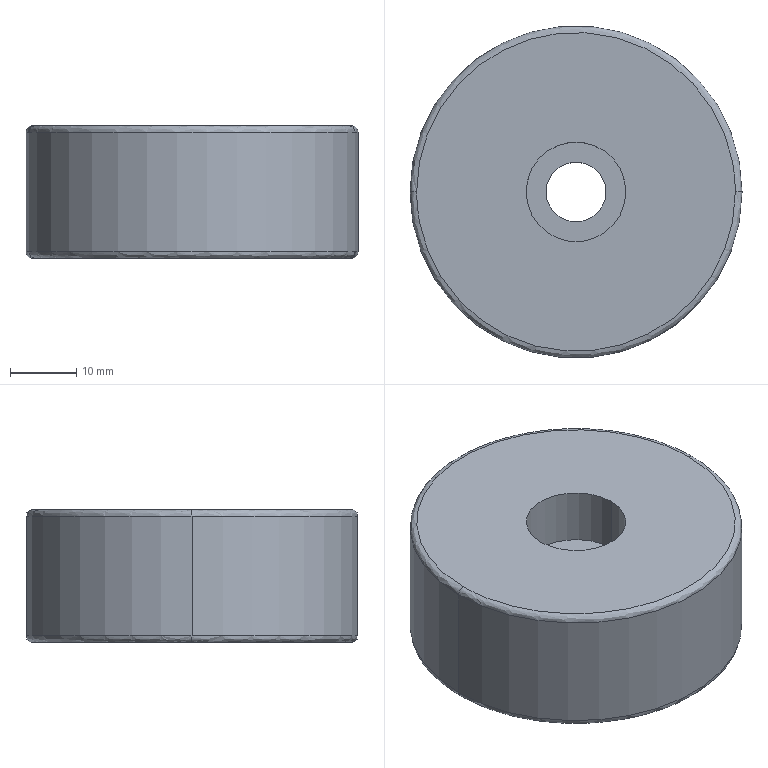Part | STEP file | Hard stop block | 1 solid | 13 faces | box 50 x 50 x 20 mm | volume 36960 mm3 | cylinder 6 | spline 4 | plane 3 | commonest cylinder face diameters 9 x2 15 x2 50 x2
STEP:
#1=CARTESIAN_POINT('',(0.,0.,0.));
#2=DIRECTION('',(0.,0.,1.));
#3=DIRECTION('',(1.,0.,0.));
#4=AXIS2_PLACEMENT_3D('',#1,#2,#3);
#5=CARTESIAN_POINT('',(25.,0.,1.));
#6=VERTEX_POINT('',#5);
#7=CARTESIAN_POINT('',(-25.,0.,1.));
#8=VERTEX_POINT('',#7);
#9=CARTESIAN_POINT('',(0.,0.,1.));
#10=DIRECTION('',(0.,0.,-1.));
#11=DIRECTION('',(1.,0.,0.));
#12=AXIS2_PLACEMENT_3D('',#9,#10,#11);
#13=CIRCLE('',#12,25.);
#14=CARTESIAN_POINT('',(-25.,0.,1.));
#15=CARTESIAN_POINT('',(-25.,-50.,1.));
#16=CARTESIAN_POINT('',(25.,-50.,1.));
#17=CARTESIAN_POINT('',(25.,0.,1.));
#18=CARTESIAN_POINT('',(-25.,0.,0.4142));
#19=CARTESIAN_POINT('',(-25.,-50.,0.4142));
#20=CARTESIAN_POINT('',(25.,-50.,0.4142));
#21=CARTESIAN_POINT('',(25.,0.,0.4142));
#22=CARTESIAN_POINT('',(-24.586,0.,0.));
#23=CARTESIAN_POINT('',(-24.586,-49.172,0.));
#24=CARTESIAN_POINT('',(24.586,-49.172,0.));
#25=CARTESIAN_POINT('',(24.586,0.,0.));
#26=CARTESIAN_POINT('',(-24.,0.,0.));
#27=CARTESIAN_POINT('',(-24.,-48.,0.));
#28=CARTESIAN_POINT('',(24.,-48.,0.));
#29=CARTESIAN_POINT('',(24.,0.,0.));
#30=(BOUNDED_SURFACE()B_SPLINE_SURFACE(3,3,((#14,#15,#16,#17),(#18,#19,#20,#21),(#22,#23,#24,#25),(#26,#27,#28,#29)),.UNSPECIFIED.,.F.,.F.,.F.)B_SPLINE_SURFACE_WITH_KNOTS((4,4),(4,4),(0.,1.),(0.,1.),.PIECEWISE_BEZIER_KNOTS.)GEOMETRIC_REPRESENTATION_ITEM()RATIONAL_B_SPLINE_SURFACE(((1.,0.3333,0.3333,1.),(0.8047,0.2682,0.2682,0.8047),(0.8047,0.2682,0.2682,0.8047),(1.,0.3333,0.3333,1.)))REPRESENTATION_ITEM('')SURFACE());
#31=CARTESIAN_POINT('',(0.,1.));
#32=CARTESIAN_POINT('',(0.,0.9763));
#33=CARTESIAN_POINT('',(0.,0.9319));
#34=CARTESIAN_POINT('',(0.,0.8733));
#35=CARTESIAN_POINT('',(0.,0.8206));
#36=CARTESIAN_POINT('',(0.,0.7724));
#37=CARTESIAN_POINT('',(0.,0.7279));
#38=CARTESIAN_POINT('',(0.,0.6861));
#39=CARTESIAN_POINT('',(0.,0.6465));
#40=CARTESIAN_POINT('',(0.,0.6086));
#41=CARTESIAN_POINT('',(0.,0.5718));
#42=CARTESIAN_POINT('',(0.,0.5357));
#43=CARTESIAN_POINT('',(0.,0.5));
#44=CARTESIAN_POINT('',(0.,0.4643));
#45=CARTESIAN_POINT('',(0.,0.4282));
#46=CARTESIAN_POINT('',(0.,0.3914));
#47=CARTESIAN_POINT('',(0.,0.3535));
#48=CARTESIAN_POINT('',(0.,0.3139));
#49=CARTESIAN_POINT('',(0.,0.2721));
#50=CARTESIAN_POINT('',(0.,0.2276));
#51=CARTESIAN_POINT('',(0.,0.1794));
#52=CARTESIAN_POINT('',(0.,0.1267));
#53=CARTESIAN_POINT('',(0.,0.06805));
#54=CARTESIAN_POINT('',(0.,0.02375));
#55=CARTESIAN_POINT('',(0.,0.));
#56=B_SPLINE_CURVE_WITH_KNOTS('',3,(#31,#32,#33,#34,#35,#36,#37,#38,#39,#40,#41,#42,#43,#44,#45,#46,#47,#48,#49,#50,#51,#52,#53,#54,#55),.UNSPECIFIED.,.F.,.F.,(4,1,1,1,1,1,1,1,1,1,1,1,1,1,1,1,1,1,1,1,1,1,4),(0.,0.1428,0.2856,0.4284,0.5712,0.714,0.8568,0.9996,1.142,1.285,1.428,1.571,1.714,1.856,1.999,2.142,2.285,2.428,2.57,2.713,2.856,2.999,3.142),.QUASI_UNIFORM_KNOTS.);
#57=(GEOMETRIC_REPRESENTATION_CONTEXT(2)PARAMETRIC_REPRESENTATION_CONTEXT()REPRESENTATION_CONTEXT('',''));
#58=DEFINITIONAL_REPRESENTATION('',(#56),#57);
#59=PCURVE('',#30,#58);
#60=CARTESIAN_POINT('',(0.,0.,20.));
#61=DIRECTION('',(0.,0.,-1.));
#62=DIRECTION('',(-1.,0.,0.));
#63=AXIS2_PLACEMENT_3D('',#60,#61,#62);
#64=CYLINDRICAL_SURFACE('',#63,25.);
#65=CARTESIAN_POINT('',(3.142,19.));
#66=DIRECTION('',(1.,0.));
#67=VECTOR('',#66,1.);
#68=LINE('',#65,#67);
#69=(GEOMETRIC_REPRESENTATION_CONTEXT(2)PARAMETRIC_REPRESENTATION_CONTEXT()REPRESENTATION_CONTEXT('',''));
#70=DEFINITIONAL_REPRESENTATION('',(#68),#69);
#71=PCURVE('',#64,#70);
#72=SURFACE_CURVE('',#13,(#59,#71),.PCURVE_S1.);
#73=EDGE_CURVE('',#6,#8,#72,.T.);
#74=ORIENTED_EDGE('',*,*,#73,.T.);
#75=CARTESIAN_POINT('',(-24.,0.,0.));
#76=VERTEX_POINT('',#75);
#77=CARTESIAN_POINT('',(-24.,0.,1.));
#78=DIRECTION('',(0.,-1.,0.));
#79=DIRECTION('',(-1.,0.,0.));
#80=AXIS2_PLACEMENT_3D('',#77,#78,#79);
#81=CIRCLE('',#80,1.);
#82=CARTESIAN_POINT('',(0.,0.));
#83=CARTESIAN_POINT('',(0.01683,0.));
#84=CARTESIAN_POINT('',(0.04999,0.));
#85=CARTESIAN_POINT('',(0.09843,0.));
#86=CARTESIAN_POINT('',(0.1457,0.));
#87=CARTESIAN_POINT('',(0.192,0.));
#88=CARTESIAN_POINT('',(0.2375,0.));
#89=CARTESIAN_POINT('',(0.2823,0.));
#90=CARTESIAN_POINT('',(0.3265,0.));
#91=CARTESIAN_POINT('',(0.3703,0.));
#92=CARTESIAN_POINT('',(0.4137,0.));
#93=CARTESIAN_POINT('',(0.4569,0.));
#94=CARTESIAN_POINT('',(0.5,0.));
#95=CARTESIAN_POINT('',(0.5431,0.));
#96=CARTESIAN_POINT('',(0.5863,0.));
#97=CARTESIAN_POINT('',(0.6297,0.));
#98=CARTESIAN_POINT('',(0.6735,0.));
#99=CARTESIAN_POINT('',(0.7177,0.));
#100=CARTESIAN_POINT('',(0.7625,0.));
#101=CARTESIAN_POINT('',(0.808,0.));
#102=CARTESIAN_POINT('',(0.8543,0.));
#103=CARTESIAN_POINT('',(0.9016,0.));
#104=CARTESIAN_POINT('',(0.95,0.));
#105=CARTESIAN_POINT('',(0.9832,0.));
#106=CARTESIAN_POINT('',(1.,0.));
#107=B_SPLINE_CURVE_WITH_KNOTS('',3,(#82,#83,#84,#85,#86,#87,#88,#89,#90,#91,#92,#93,#94,#95,#96,#97,#98,#99,#100,#101,#102,#103,#104,#105,#106),.UNSPECIFIED.,.F.,.F.,(4,1,1,1,1,1,1,1,1,1,1,1,1,1,1,1,1,1,1,1,1,1,4),(0.,0.0714,0.1428,0.2142,0.2856,0.357,0.4284,0.4998,0.5712,0.6426,0.714,0.7854,0.8568,0.9282,0.9996,1.071,1.142,1.214,1.285,1.357,1.428,1.499,1.571),.QUASI_UNIFORM_KNOTS.);
#108=(GEOMETRIC_REPRESENTATION_CONTEXT(2)PARAMETRIC_REPRESENTATION_CONTEXT()REPRESENTATION_CONTEXT('',''));
#109=DEFINITIONAL_REPRESENTATION('',(#107),#108);
#110=PCURVE('',#30,#109);
#111=CARTESIAN_POINT('',(25.,0.,1.));
#112=CARTESIAN_POINT('',(25.,50.,1.));
#113=CARTESIAN_POINT('',(-25.,50.,1.));
#114=CARTESIAN_POINT('',(-25.,0.,1.));
#115=CARTESIAN_POINT('',(25.,0.,0.4142));
#116=CARTESIAN_POINT('',(25.,50.,0.4142));
#117=CARTESIAN_POINT('',(-25.,50.,0.4142));
#118=CARTESIAN_POINT('',(-25.,0.,0.4142));
#119=CARTESIAN_POINT('',(24.586,0.,0.));
#120=CARTESIAN_POINT('',(24.586,49.172,0.));
#121=CARTESIAN_POINT('',(-24.586,49.172,0.));
#122=CARTESIAN_POINT('',(-24.586,0.,0.));
#123=CARTESIAN_POINT('',(24.,0.,0.));
#124=CARTESIAN_POINT('',(24.,48.,0.));
#125=CARTESIAN_POINT('',(-24.,48.,0.));
#126=CARTESIAN_POINT('',(-24.,0.,0.));
#127=(BOUNDED_SURFACE()B_SPLINE_SURFACE(3,3,((#111,#112,#113,#114),(#115,#116,#117,#118),(#119,#120,#121,#122),(#123,#124,#125,#126)),.UNSPECIFIED.,.F.,.F.,.F.)B_SPLINE_SURFACE_WITH_KNOTS((4,4),(4,4),(0.,1.),(0.,1.),.PIECEWISE_BEZIER_KNOTS.)GEOMETRIC_REPRESENTATION_ITEM()RATIONAL_B_SPLINE_SURFACE(((1.,0.3333,0.3333,1.),(0.8047,0.2682,0.2682,0.8047),(0.8047,0.2682,0.2682,0.8047),(1.,0.3333,0.3333,1.)))REPRESENTATION_ITEM('')SURFACE());
#128=CARTESIAN_POINT('',(0.,1.));
#129=CARTESIAN_POINT('',(0.01683,1.));
#130=CARTESIAN_POINT('',(0.04999,1.));
#131=CARTESIAN_POINT('',(0.09843,1.));
#132=CARTESIAN_POINT('',(0.1457,1.));
#133=CARTESIAN_POINT('',(0.192,1.));
#134=CARTESIAN_POINT('',(0.2375,1.));
#135=CARTESIAN_POINT('',(0.2823,1.));
#136=CARTESIAN_POINT('',(0.3265,1.));
#137=CARTESIAN_POINT('',(0.3703,1.));
#138=CARTESIAN_POINT('',(0.4137,1.));
#139=CARTESIAN_POINT('',(0.4569,1.));
#140=CARTESIAN_POINT('',(0.5,1.));
#141=CARTESIAN_POINT('',(0.5431,1.));
#142=CARTESIAN_POINT('',(0.5863,1.));
#143=CARTESIAN_POINT('',(0.6297,1.));
#144=CARTESIAN_POINT('',(0.6735,1.));
#145=CARTESIAN_POINT('',(0.7177,1.));
#146=CARTESIAN_POINT('',(0.7625,1.));
#147=CARTESIAN_POINT('',(0.808,1.));
#148=CARTESIAN_POINT('',(0.8543,1.));
#149=CARTESIAN_POINT('',(0.9016,1.));
#150=CARTESIAN_POINT('',(0.95,1.));
#151=CARTESIAN_POINT('',(0.9832,1.));
#152=CARTESIAN_POINT('',(1.,1.));
#153=B_SPLINE_CURVE_WITH_KNOTS('',3,(#128,#129,#130,#131,#132,#133,#134,#135,#136,#137,#138,#139,#140,#141,#142,#143,#144,#145,#146,#147,#148,#149,#150,#151,#152),.UNSPECIFIED.,.F.,.F.,(4,1,1,1,1,1,1,1,1,1,1,1,1,1,1,1,1,1,1,1,1,1,4),(0.,0.0714,0.1428,0.2142,0.2856,0.357,0.4284,0.4998,0.5712,0.6426,0.714,0.7854,0.8568,0.9282,0.9996,1.071,1.142,1.214,1.285,1.357,1.428,1.499,1.571),.QUASI_UNIFORM_KNOTS.);
#154=(GEOMETRIC_REPRESENTATION_CONTEXT(2)PARAMETRIC_REPRESENTATION_CONTEXT()REPRESENTATION_CONTEXT('',''));
#155=DEFINITIONAL_REPRESENTATION('',(#153),#154);
#156=PCURVE('',#127,#155);
#157=SURFACE_CURVE('',#81,(#110,#156),.PCURVE_S1.);
#158=EDGE_CURVE('',#8,#76,#157,.T.);
#159=ORIENTED_EDGE('',*,*,#158,.T.);
#160=CARTESIAN_POINT('',(24.,0.,0.));
#161=VERTEX_POINT('',#160);
#162=CARTESIAN_POINT('',(-24.,0.,0.));
#163=CARTESIAN_POINT('',(-24.,-48.,0.));
#164=CARTESIAN_POINT('',(24.,-48.,0.));
#165=CARTESIAN_POINT('',(24.,0.,0.));
#166=(BOUNDED_CURVE()B_SPLINE_CURVE(3,(#162,#163,#164,#165),.UNSPECIFIED.,.F.,.F.)B_SPLINE_CURVE_WITH_KNOTS((4,4),(0.,1.),.PIECEWISE_BEZIER_KNOTS.)CURVE()GEOMETRIC_REPRESENTATION_ITEM()RATIONAL_B_SPLINE_CURVE((1.,0.3333,0.3333,1.))REPRESENTATION_ITEM(''));
#167=CARTESIAN_POINT('',(1.,0.));
#168=DIRECTION('',(0.,1.));
#169=VECTOR('',#168,1.);
#170=LINE('',#167,#169);
#171=(GEOMETRIC_REPRESENTATION_CONTEXT(2)PARAMETRIC_REPRESENTATION_CONTEXT()REPRESENTATION_CONTEXT('',''));
#172=DEFINITIONAL_REPRESENTATION('',(#170),#171);
#173=PCURVE('',#30,#172);
#174=CARTESIAN_POINT('',(0.,0.,0.));
#175=DIRECTION('',(0.,0.,1.));
#176=DIRECTION('',(1.,0.,0.));
#177=AXIS2_PLACEMENT_3D('',#174,#175,#176);
#178=PLANE('',#177);
#179=CARTESIAN_POINT('',(-24.,0.));
#180=CARTESIAN_POINT('',(-24.,-48.));
#181=CARTESIAN_POINT('',(24.,-48.));
#182=CARTESIAN_POINT('',(24.,0.));
#183=(BOUNDED_CURVE()B_SPLINE_CURVE(3,(#179,#180,#181,#182),.UNSPECIFIED.,.F.,.F.)B_SPLINE_CURVE_WITH_KNOTS((4,4),(0.,1.),.PIECEWISE_BEZIER_KNOTS.)CURVE()GEOMETRIC_REPRESENTATION_ITEM()RATIONAL_B_SPLINE_CURVE((1.,0.3333,0.3333,1.))REPRESENTATION_ITEM(''));
#184=(GEOMETRIC_REPRESENTATION_CONTEXT(2)PARAMETRIC_REPRESENTATION_CONTEXT()REPRESENTATION_CONTEXT('',''));
#185=DEFINITIONAL_REPRESENTATION('',(#183),#184);
#186=PCURVE('',#178,#185);
#187=SURFACE_CURVE('',#166,(#173,#186),.PCURVE_S1.);
#188=EDGE_CURVE('',#76,#161,#187,.T.);
#189=ORIENTED_EDGE('',*,*,#188,.T.);
#190=CARTESIAN_POINT('',(24.,0.,1.));
#191=DIRECTION('',(0.,1.,0.));
#192=DIRECTION('',(1.,0.,0.));
#193=AXIS2_PLACEMENT_3D('',#190,#191,#192);
#194=CIRCLE('',#193,1.);
#195=CARTESIAN_POINT('',(0.,1.));
#196=CARTESIAN_POINT('',(0.01683,1.));
#197=CARTESIAN_POINT('',(0.04999,1.));
#198=CARTESIAN_POINT('',(0.09843,1.));
#199=CARTESIAN_POINT('',(0.1457,1.));
#200=CARTESIAN_POINT('',(0.192,1.));
#201=CARTESIAN_POINT('',(0.2375,1.));
#202=CARTESIAN_POINT('',(0.2823,1.));
#203=CARTESIAN_POINT('',(0.3265,1.));
#204=CARTESIAN_POINT('',(0.3703,1.));
#205=CARTESIAN_POINT('',(0.4137,1.));
#206=CARTESIAN_POINT('',(0.4569,1.));
#207=CARTESIAN_POINT('',(0.5,1.));
#208=CARTESIAN_POINT('',(0.5431,1.));
#209=CARTESIAN_POINT('',(0.5863,1.));
#210=CARTESIAN_POINT('',(0.6297,1.));
#211=CARTESIAN_POINT('',(0.6735,1.));
#212=CARTESIAN_POINT('',(0.7177,1.));
#213=CARTESIAN_POINT('',(0.7625,1.));
#214=CARTESIAN_POINT('',(0.808,1.));
#215=CARTESIAN_POINT('',(0.8543,1.));
#216=CARTESIAN_POINT('',(0.9016,1.));
#217=CARTESIAN_POINT('',(0.95,1.));
#218=CARTESIAN_POINT('',(0.9832,1.));
#219=CARTESIAN_POINT('',(1.,1.));
#220=B_SPLINE_CURVE_WITH_KNOTS('',3,(#195,#196,#197,#198,#199,#200,#201,#202,#203,#204,#205,#206,#207,#208,#209,#210,#211,#212,#213,#214,#215,#216,#217,#218,#219),.UNSPECIFIED.,.F.,.F.,(4,1,1,1,1,1,1,1,1,1,1,1,1,1,1,1,1,1,1,1,1,1,4),(0.,0.0714,0.1428,0.2142,0.2856,0.357,0.4284,0.4998,0.5712,0.6426,0.714,0.7854,0.8568,0.9282,0.9996,1.071,1.142,1.214,1.285,1.357,1.428,1.499,1.571),.QUASI_UNIFORM_KNOTS.);
#221=(GEOMETRIC_REPRESENTATION_CONTEXT(2)PARAMETRIC_REPRESENTATION_CONTEXT()REPRESENTATION_CONTEXT('',''));
#222=DEFINITIONAL_REPRESENTATION('',(#220),#221);
#223=PCURVE('',#30,#222);
#224=CARTESIAN_POINT('',(0.,0.));
#225=CARTESIAN_POINT('',(0.01683,0.));
#226=CARTESIAN_POINT('',(0.04999,0.));
#227=CARTESIAN_POINT('',(0.09843,0.));
#228=CARTESIAN_POINT('',(0.1457,0.));
#229=CARTESIAN_POINT('',(0.192,0.));
#230=CARTESIAN_POINT('',(0.2375,0.));
#231=CARTESIAN_POINT('',(0.2823,0.));
#232=CARTESIAN_POINT('',(0.3265,0.));
#233=CARTESIAN_POINT('',(0.3703,0.));
#234=CARTESIAN_POINT('',(0.4137,0.));
#235=CARTESIAN_POINT('',(0.4569,0.));
#236=CARTESIAN_POINT('',(0.5,0.));
#237=CARTESIAN_POINT('',(0.5431,0.));
#238=CARTESIAN_POINT('',(0.5863,0.));
#239=CARTESIAN_POINT('',(0.6297,0.));
#240=CARTESIAN_POINT('',(0.6735,0.));
#241=CARTESIAN_POINT('',(0.7177,0.));
#242=CARTESIAN_POINT('',(0.7625,0.));
#243=CARTESIAN_POINT('',(0.808,0.));
#244=CARTESIAN_POINT('',(0.8543,0.));
#245=CARTESIAN_POINT('',(0.9016,0.));
#246=CARTESIAN_POINT('',(0.95,0.));
#247=CARTESIAN_POINT('',(0.9832,0.));
#248=CARTESIAN_POINT('',(1.,0.));
#249=B_SPLINE_CURVE_WITH_KNOTS('',3,(#224,#225,#226,#227,#228,#229,#230,#231,#232,#233,#234,#235,#236,#237,#238,#239,#240,#241,#242,#243,#244,#245,#246,#247,#248),.UNSPECIFIED.,.F.,.F.,(4,1,1,1,1,1,1,1,1,1,1,1,1,1,1,1,1,1,1,1,1,1,4),(0.,0.0714,0.1428,0.2142,0.2856,0.357,0.4284,0.4998,0.5712,0.6426,0.714,0.7854,0.8568,0.9282,0.9996,1.071,1.142,1.214,1.285,1.357,1.428,1.499,1.571),.QUASI_UNIFORM_KNOTS.);
#250=(GEOMETRIC_REPRESENTATION_CONTEXT(2)PARAMETRIC_REPRESENTATION_CONTEXT()REPRESENTATION_CONTEXT('',''));
#251=DEFINITIONAL_REPRESENTATION('',(#249),#250);
#252=PCURVE('',#127,#251);
#253=SURFACE_CURVE('',#194,(#223,#252),.PCURVE_S1.);
#254=EDGE_CURVE('',#6,#161,#253,.T.);
#255=ORIENTED_EDGE('',*,*,#254,.F.);
#256=EDGE_LOOP('',(#74,#159,#189,#255));
#257=FACE_BOUND('',#256,.T.);
#258=ADVANCED_FACE('',(#257),#30,.T.);
#259=CARTESIAN_POINT('',(24.,0.,20.));
#260=VERTEX_POINT('',#259);
#261=CARTESIAN_POINT('',(-24.,0.,20.));
#262=VERTEX_POINT('',#261);
#263=CARTESIAN_POINT('',(24.,0.,20.));
#264=CARTESIAN_POINT('',(24.,-48.,20.));
#265=CARTESIAN_POINT('',(-24.,-48.,20.));
#266=CARTESIAN_POINT('',(-24.,0.,20.));
#267=(BOUNDED_CURVE()B_SPLINE_CURVE(3,(#263,#264,#265,#266),.UNSPECIFIED.,.F.,.F.)B_SPLINE_CURVE_WITH_KNOTS((4,4),(0.,1.),.PIECEWISE_BEZIER_KNOTS.)CURVE()GEOMETRIC_REPRESENTATION_ITEM()RATIONAL_B_SPLINE_CURVE((1.,0.3333,0.3333,1.))REPRESENTATION_ITEM(''));
#268=CARTESIAN_POINT('',(-24.,0.,20.));
#269=CARTESIAN_POINT('',(-24.,-48.,20.));
#270=CARTESIAN_POINT('',(24.,-48.,20.));
#271=CARTESIAN_POINT('',(24.,0.,20.));
#272=CARTESIAN_POINT('',(-24.586,0.,20.));
#273=CARTESIAN_POINT('',(-24.586,-49.172,20.));
#274=CARTESIAN_POINT('',(24.586,-49.172,20.));
#275=CARTESIAN_POINT('',(24.586,0.,20.));
#276=CARTESIAN_POINT('',(-25.,0.,19.586));
#277=CARTESIAN_POINT('',(-25.,-50.,19.586));
#278=CARTESIAN_POINT('',(25.,-50.,19.586));
#279=CARTESIAN_POINT('',(25.,0.,19.586));
#280=CARTESIAN_POINT('',(-25.,0.,19.));
#281=CARTESIAN_POINT('',(-25.,-50.,19.));
#282=CARTESIAN_POINT('',(25.,-50.,19.));
#283=CARTESIAN_POINT('',(25.,0.,19.));
#284=(BOUNDED_SURFACE()B_SPLINE_SURFACE(3,3,((#268,#269,#270,#271),(#272,#273,#274,#275),(#276,#277,#278,#279),(#280,#281,#282,#283)),.UNSPECIFIED.,.F.,.F.,.F.)B_SPLINE_SURFACE_WITH_KNOTS((4,4),(4,4),(0.,1.),(0.,1.),.PIECEWISE_BEZIER_KNOTS.)GEOMETRIC_REPRESENTATION_ITEM()RATIONAL_B_SPLINE_SURFACE(((1.,0.3333,0.3333,1.),(0.8047,0.2682,0.2682,0.8047),(0.8047,0.2682,0.2682,0.8047),(1.,0.3333,0.3333,1.)))REPRESENTATION_ITEM('')SURFACE());
#285=CARTESIAN_POINT('',(0.,1.));
#286=DIRECTION('',(0.,-1.));
#287=VECTOR('',#286,1.);
#288=LINE('',#285,#287);
#289=(GEOMETRIC_REPRESENTATION_CONTEXT(2)PARAMETRIC_REPRESENTATION_CONTEXT()REPRESENTATION_CONTEXT('',''));
#290=DEFINITIONAL_REPRESENTATION('',(#288),#289);
#291=PCURVE('',#284,#290);
#292=CARTESIAN_POINT('',(0.,0.,20.));
#293=DIRECTION('',(0.,0.,1.));
#294=DIRECTION('',(1.,0.,0.));
#295=AXIS2_PLACEMENT_3D('',#292,#293,#294);
#296=PLANE('',#295);
#297=CARTESIAN_POINT('',(24.,0.));
#298=CARTESIAN_POINT('',(24.,-48.));
#299=CARTESIAN_POINT('',(-24.,-48.));
#300=CARTESIAN_POINT('',(-24.,0.));
#301=(BOUNDED_CURVE()B_SPLINE_CURVE(3,(#297,#298,#299,#300),.UNSPECIFIED.,.F.,.F.)B_SPLINE_CURVE_WITH_KNOTS((4,4),(0.,1.),.PIECEWISE_BEZIER_KNOTS.)CURVE()GEOMETRIC_REPRESENTATION_ITEM()RATIONAL_B_SPLINE_CURVE((1.,0.3333,0.3333,1.))REPRESENTATION_ITEM(''));
#302=(GEOMETRIC_REPRESENTATION_CONTEXT(2)PARAMETRIC_REPRESENTATION_CONTEXT()REPRESENTATION_CONTEXT('',''));
#303=DEFINITIONAL_REPRESENTATION('',(#301),#302);
#304=PCURVE('',#296,#303);
#305=SURFACE_CURVE('',#267,(#291,#304),.PCURVE_S1.);
#306=EDGE_CURVE('',#260,#262,#305,.T.);
#307=ORIENTED_EDGE('',*,*,#306,.T.);
#308=CARTESIAN_POINT('',(-25.,0.,19.));
#309=VERTEX_POINT('',#308);
#310=CARTESIAN_POINT('',(-24.,0.,19.));
#311=DIRECTION('',(0.,-1.,0.));
#312=DIRECTION('',(-1.,0.,0.));
#313=AXIS2_PLACEMENT_3D('',#310,#311,#312);
#314=CIRCLE('',#313,1.);
#315=CARTESIAN_POINT('',(0.,0.));
#316=CARTESIAN_POINT('',(0.01683,0.));
#317=CARTESIAN_POINT('',(0.04999,0.));
#318=CARTESIAN_POINT('',(0.09843,0.));
#319=CARTESIAN_POINT('',(0.1457,0.));
#320=CARTESIAN_POINT('',(0.192,0.));
#321=CARTESIAN_POINT('',(0.2375,0.));
#322=CARTESIAN_POINT('',(0.2823,0.));
#323=CARTESIAN_POINT('',(0.3265,0.));
#324=CARTESIAN_POINT('',(0.3703,0.));
#325=CARTESIAN_POINT('',(0.4137,0.));
#326=CARTESIAN_POINT('',(0.4569,0.));
#327=CARTESIAN_POINT('',(0.5,0.));
#328=CARTESIAN_POINT('',(0.5431,0.));
#329=CARTESIAN_POINT('',(0.5863,0.));
#330=CARTESIAN_POINT('',(0.6297,0.));
#331=CARTESIAN_POINT('',(0.6735,0.));
#332=CARTESIAN_POINT('',(0.7177,0.));
#333=CARTESIAN_POINT('',(0.7625,0.));
#334=CARTESIAN_POINT('',(0.808,0.));
#335=CARTESIAN_POINT('',(0.8543,0.));
#336=CARTESIAN_POINT('',(0.9016,0.));
#337=CARTESIAN_POINT('',(0.95,0.));
#338=CARTESIAN_POINT('',(0.9832,0.));
#339=CARTESIAN_POINT('',(1.,0.));
#340=B_SPLINE_CURVE_WITH_KNOTS('',3,(#315,#316,#317,#318,#319,#320,#321,#322,#323,#324,#325,#326,#327,#328,#329,#330,#331,#332,#333,#334,#335,#336,#337,#338,#339),.UNSPECIFIED.,.F.,.F.,(4,1,1,1,1,1,1,1,1,1,1,1,1,1,1,1,1,1,1,1,1,1,4),(4.712,4.784,4.855,4.927,4.998,5.069,5.141,5.212,5.284,5.355,5.426,5.498,5.569,5.641,5.712,5.783,5.855,5.926,5.998,6.069,6.14,6.212,6.283),.QUASI_UNIFORM_KNOTS.);
#341=(GEOMETRIC_REPRESENTATION_CONTEXT(2)PARAMETRIC_REPRESENTATION_CONTEXT()REPRESENTATION_CONTEXT('',''));
#342=DEFINITIONAL_REPRESENTATION('',(#340),#341);
#343=PCURVE('',#284,#342);
#344=CARTESIAN_POINT('',(24.,0.,20.));
#345=CARTESIAN_POINT('',(24.,48.,20.));
#346=CARTESIAN_POINT('',(-24.,48.,20.));
#347=CARTESIAN_POINT('',(-24.,0.,20.));
#348=CARTESIAN_POINT('',(24.586,0.,20.));
#349=CARTESIAN_POINT('',(24.586,49.172,20.));
#350=CARTESIAN_POINT('',(-24.586,49.172,20.));
#351=CARTESIAN_POINT('',(-24.586,0.,20.));
#352=CARTESIAN_POINT('',(25.,0.,19.586));
#353=CARTESIAN_POINT('',(25.,50.,19.586));
#354=CARTESIAN_POINT('',(-25.,50.,19.586));
#355=CARTESIAN_POINT('',(-25.,0.,19.586));
#356=CARTESIAN_POINT('',(25.,0.,19.));
#357=CARTESIAN_POINT('',(25.,50.,19.));
#358=CARTESIAN_POINT('',(-25.,50.,19.));
#359=CARTESIAN_POINT('',(-25.,0.,19.));
#360=(BOUNDED_SURFACE()B_SPLINE_SURFACE(3,3,((#344,#345,#346,#347),(#348,#349,#350,#351),(#352,#353,#354,#355),(#356,#357,#358,#359)),.UNSPECIFIED.,.F.,.F.,.F.)B_SPLINE_SURFACE_WITH_KNOTS((4,4),(4,4),(0.,1.),(0.,1.),.PIECEWISE_BEZIER_KNOTS.)GEOMETRIC_REPRESENTATION_ITEM()RATIONAL_B_SPLINE_SURFACE(((1.,0.3333,0.3333,1.),(0.8047,0.2682,0.2682,0.8047),(0.8047,0.2682,0.2682,0.8047),(1.,0.3333,0.3333,1.)))REPRESENTATION_ITEM('')SURFACE());
#361=CARTESIAN_POINT('',(0.,1.));
#362=CARTESIAN_POINT('',(0.01683,1.));
#363=CARTESIAN_POINT('',(0.04999,1.));
#364=CARTESIAN_POINT('',(0.09843,1.));
#365=CARTESIAN_POINT('',(0.1457,1.));
#366=CARTESIAN_POINT('',(0.192,1.));
#367=CARTESIAN_POINT('',(0.2375,1.));
#368=CARTESIAN_POINT('',(0.2823,1.));
#369=CARTESIAN_POINT('',(0.3265,1.));
#370=CARTESIAN_POINT('',(0.3703,1.));
#371=CARTESIAN_POINT('',(0.4137,1.));
#372=CARTESIAN_POINT('',(0.4569,1.));
#373=CARTESIAN_POINT('',(0.5,1.));
#374=CARTESIAN_POINT('',(0.5431,1.));
#375=CARTESIAN_POINT('',(0.5863,1.));
#376=CARTESIAN_POINT('',(0.6297,1.));
#377=CARTESIAN_POINT('',(0.6735,1.));
#378=CARTESIAN_POINT('',(0.7177,1.));
#379=CARTESIAN_POINT('',(0.7625,1.));
#380=CARTESIAN_POINT('',(0.808,1.));
#381=CARTESIAN_POINT('',(0.8543,1.));
#382=CARTESIAN_POINT('',(0.9016,1.));
#383=CARTESIAN_POINT('',(0.95,1.));
#384=CARTESIAN_POINT('',(0.9832,1.));
#385=CARTESIAN_POINT('',(1.,1.));
#386=B_SPLINE_CURVE_WITH_KNOTS('',3,(#361,#362,#363,#364,#365,#366,#367,#368,#369,#370,#371,#372,#373,#374,#375,#376,#377,#378,#379,#380,#381,#382,#383,#384,#385),.UNSPECIFIED.,.F.,.F.,(4,1,1,1,1,1,1,1,1,1,1,1,1,1,1,1,1,1,1,1,1,1,4),(4.712,4.784,4.855,4.927,4.998,5.069,5.141,5.212,5.284,5.355,5.426,5.498,5.569,5.641,5.712,5.783,5.855,5.926,5.998,6.069,6.14,6.212,6.283),.QUASI_UNIFORM_KNOTS.);
#387=(GEOMETRIC_REPRESENTATION_CONTEXT(2)PARAMETRIC_REPRESENTATION_CONTEXT()REPRESENTATION_CONTEXT('',''));
#388=DEFINITIONAL_REPRESENTATION('',(#386),#387);
#389=PCURVE('',#360,#388);
#390=SURFACE_CURVE('',#314,(#343,#389),.PCURVE_S1.);
#391=EDGE_CURVE('',#262,#309,#390,.T.);
#392=ORIENTED_EDGE('',*,*,#391,.T.);
#393=CARTESIAN_POINT('',(25.,0.,19.));
#394=VERTEX_POINT('',#393);
#395=CARTESIAN_POINT('',(0.,0.,19.));
#396=DIRECTION('',(0.,0.,-1.));
#397=DIRECTION('',(-1.,0.,0.));
#398=AXIS2_PLACEMENT_3D('',#395,#396,#397);
#399=CIRCLE('',#398,25.);
#400=CARTESIAN_POINT('',(1.,1.));
#401=CARTESIAN_POINT('',(1.,0.9763));
#402=CARTESIAN_POINT('',(1.,0.9319));
#403=CARTESIAN_POINT('',(1.,0.8733));
#404=CARTESIAN_POINT('',(1.,0.8206));
#405=CARTESIAN_POINT('',(1.,0.7724));
#406=CARTESIAN_POINT('',(1.,0.7279));
#407=CARTESIAN_POINT('',(1.,0.6861));
#408=CARTESIAN_POINT('',(1.,0.6465));
#409=CARTESIAN_POINT('',(1.,0.6086));
#410=CARTESIAN_POINT('',(1.,0.5718));
#411=CARTESIAN_POINT('',(1.,0.5357));
#412=CARTESIAN_POINT('',(1.,0.5));
#413=CARTESIAN_POINT('',(1.,0.4643));
#414=CARTESIAN_POINT('',(1.,0.4282));
#415=CARTESIAN_POINT('',(1.,0.3914));
#416=CARTESIAN_POINT('',(1.,0.3535));
#417=CARTESIAN_POINT('',(1.,0.3139));
#418=CARTESIAN_POINT('',(1.,0.2721));
#419=CARTESIAN_POINT('',(1.,0.2276));
#420=CARTESIAN_POINT('',(1.,0.1794));
#421=CARTESIAN_POINT('',(1.,0.1267));
#422=CARTESIAN_POINT('',(1.,0.06805));
#423=CARTESIAN_POINT('',(1.,0.02375));
#424=CARTESIAN_POINT('',(1.,0.));
#425=B_SPLINE_CURVE_WITH_KNOTS('',3,(#400,#401,#402,#403,#404,#405,#406,#407,#408,#409,#410,#411,#412,#413,#414,#415,#416,#417,#418,#419,#420,#421,#422,#423,#424),.UNSPECIFIED.,.F.,.F.,(4,1,1,1,1,1,1,1,1,1,1,1,1,1,1,1,1,1,1,1,1,1,4),(3.142,3.284,3.427,3.57,3.713,3.856,3.998,4.141,4.284,4.427,4.57,4.712,4.855,4.998,5.141,5.284,5.426,5.569,5.712,5.855,5.998,6.14,6.283),.QUASI_UNIFORM_KNOTS.);
#426=(GEOMETRIC_REPRESENTATION_CONTEXT(2)PARAMETRIC_REPRESENTATION_CONTEXT()REPRESENTATION_CONTEXT('',''));
#427=DEFINITIONAL_REPRESENTATION('',(#425),#426);
#428=PCURVE('',#284,#427);
#429=CARTESIAN_POINT('',(0.,1.));
#430=DIRECTION('',(1.,0.));
#431=VECTOR('',#430,1.);
#432=LINE('',#429,#431);
#433=(GEOMETRIC_REPRESENTATION_CONTEXT(2)PARAMETRIC_REPRESENTATION_CONTEXT()REPRESENTATION_CONTEXT('',''));
#434=DEFINITIONAL_REPRESENTATION('',(#432),#433);
#435=PCURVE('',#64,#434);
#436=SURFACE_CURVE('',#399,(#428,#435),.PCURVE_S1.);
#437=EDGE_CURVE('',#394,#309,#436,.T.);
#438=ORIENTED_EDGE('',*,*,#437,.F.);
#439=CARTESIAN_POINT('',(24.,0.,19.));
#440=DIRECTION('',(0.,1.,0.));
#441=DIRECTION('',(1.,0.,0.));
#442=AXIS2_PLACEMENT_3D('',#439,#440,#441);
#443=CIRCLE('',#442,1.);
#444=CARTESIAN_POINT('',(0.,1.));
#445=CARTESIAN_POINT('',(0.01683,1.));
#446=CARTESIAN_POINT('',(0.04999,1.));
#447=CARTESIAN_POINT('',(0.09843,1.));
#448=CARTESIAN_POINT('',(0.1457,1.));
#449=CARTESIAN_POINT('',(0.192,1.));
#450=CARTESIAN_POINT('',(0.2375,1.));
#451=CARTESIAN_POINT('',(0.2823,1.));
#452=CARTESIAN_POINT('',(0.3265,1.));
#453=CARTESIAN_POINT('',(0.3703,1.));
#454=CARTESIAN_POINT('',(0.4137,1.));
#455=CARTESIAN_POINT('',(0.4569,1.));
#456=CARTESIAN_POINT('',(0.5,1.));
#457=CARTESIAN_POINT('',(0.5431,1.));
#458=CARTESIAN_POINT('',(0.5863,1.));
#459=CARTESIAN_POINT('',(0.6297,1.));
#460=CARTESIAN_POINT('',(0.6735,1.));
#461=CARTESIAN_POINT('',(0.7177,1.));
#462=CARTESIAN_POINT('',(0.7625,1.));
#463=CARTESIAN_POINT('',(0.808,1.));
#464=CARTESIAN_POINT('',(0.8543,1.));
#465=CARTESIAN_POINT('',(0.9016,1.));
#466=CARTESIAN_POINT('',(0.95,1.));
#467=CARTESIAN_POINT('',(0.9832,1.));
#468=CARTESIAN_POINT('',(1.,1.));
#469=B_SPLINE_CURVE_WITH_KNOTS('',3,(#444,#445,#446,#447,#448,#449,#450,#451,#452,#453,#454,#455,#456,#457,#458,#459,#460,#461,#462,#463,#464,#465,#466,#467,#468),.UNSPECIFIED.,.F.,.F.,(4,1,1,1,1,1,1,1,1,1,1,1,1,1,1,1,1,1,1,1,1,1,4),(4.712,4.784,4.855,4.927,4.998,5.069,5.141,5.212,5.284,5.355,5.426,5.498,5.569,5.641,5.712,5.783,5.855,5.926,5.998,6.069,6.14,6.212,6.283),.QUASI_UNIFORM_KNOTS.);
#470=(GEOMETRIC_REPRESENTATION_CONTEXT(2)PARAMETRIC_REPRESENTATION_CONTEXT()REPRESENTATION_CONTEXT('',''));
#471=DEFINITIONAL_REPRESENTATION('',(#469),#470);
#472=PCURVE('',#284,#471);
#473=CARTESIAN_POINT('',(0.,0.));
#474=CARTESIAN_POINT('',(0.01683,0.));
#475=CARTESIAN_POINT('',(0.04999,0.));
#476=CARTESIAN_POINT('',(0.09843,0.));
#477=CARTESIAN_POINT('',(0.1457,0.));
#478=CARTESIAN_POINT('',(0.192,0.));
#479=CARTESIAN_POINT('',(0.2375,0.));
#480=CARTESIAN_POINT('',(0.2823,0.));
#481=CARTESIAN_POINT('',(0.3265,0.));
#482=CARTESIAN_POINT('',(0.3703,0.));
#483=CARTESIAN_POINT('',(0.4137,0.));
#484=CARTESIAN_POINT('',(0.4569,0.));
#485=CARTESIAN_POINT('',(0.5,0.));
#486=CARTESIAN_POINT('',(0.5431,0.));
#487=CARTESIAN_POINT('',(0.5863,0.));
#488=CARTESIAN_POINT('',(0.6297,0.));
#489=CARTESIAN_POINT('',(0.6735,0.));
#490=CARTESIAN_POINT('',(0.7177,0.));
#491=CARTESIAN_POINT('',(0.7625,0.));
#492=CARTESIAN_POINT('',(0.808,0.));
#493=CARTESIAN_POINT('',(0.8543,0.));
#494=CARTESIAN_POINT('',(0.9016,0.));
#495=CARTESIAN_POINT('',(0.95,0.));
#496=CARTESIAN_POINT('',(0.9832,0.));
#497=CARTESIAN_POINT('',(1.,0.));
#498=B_SPLINE_CURVE_WITH_KNOTS('',3,(#473,#474,#475,#476,#477,#478,#479,#480,#481,#482,#483,#484,#485,#486,#487,#488,#489,#490,#491,#492,#493,#494,#495,#496,#497),.UNSPECIFIED.,.F.,.F.,(4,1,1,1,1,1,1,1,1,1,1,1,1,1,1,1,1,1,1,1,1,1,4),(4.712,4.784,4.855,4.927,4.998,5.069,5.141,5.212,5.284,5.355,5.426,5.498,5.569,5.641,5.712,5.783,5.855,5.926,5.998,6.069,6.14,6.212,6.283),.QUASI_UNIFORM_KNOTS.);
#499=(GEOMETRIC_REPRESENTATION_CONTEXT(2)PARAMETRIC_REPRESENTATION_CONTEXT()REPRESENTATION_CONTEXT('',''));
#500=DEFINITIONAL_REPRESENTATION('',(#498),#499);
#501=PCURVE('',#360,#500);
#502=SURFACE_CURVE('',#443,(#472,#501),.PCURVE_S1.);
#503=EDGE_CURVE('',#260,#394,#502,.T.);
#504=ORIENTED_EDGE('',*,*,#503,.F.);
#505=EDGE_LOOP('',(#307,#392,#438,#504));
#506=FACE_BOUND('',#505,.T.);
#507=ADVANCED_FACE('',(#506),#284,.T.);
#508=CARTESIAN_POINT('',(4.5,0.,0.));
#509=VERTEX_POINT('',#508);
#510=CARTESIAN_POINT('',(4.5,0.,11.4));
#511=VERTEX_POINT('',#510);
#512=CARTESIAN_POINT('',(4.5,0.,20.));
#513=DIRECTION('',(0.,0.,1.));
#514=VECTOR('',#513,1.);
#515=LINE('',#512,#514);
#516=CARTESIAN_POINT('',(0.,0.,20.));
#517=DIRECTION('',(0.,0.,1.));
#518=DIRECTION('',(1.,0.,0.));
#519=AXIS2_PLACEMENT_3D('',#516,#517,#518);
#520=CYLINDRICAL_SURFACE('',#519,4.5);
#521=CARTESIAN_POINT('',(6.283,0.));
#522=DIRECTION('',(0.,1.));
#523=VECTOR('',#522,1.);
#524=LINE('',#521,#523);
#525=(GEOMETRIC_REPRESENTATION_CONTEXT(2)PARAMETRIC_REPRESENTATION_CONTEXT()REPRESENTATION_CONTEXT('',''));
#526=DEFINITIONAL_REPRESENTATION('',(#524),#525);
#527=PCURVE('',#520,#526);
#528=CARTESIAN_POINT('',(0.,0.,20.));
#529=DIRECTION('',(0.,0.,1.));
#530=DIRECTION('',(1.,0.,0.));
#531=AXIS2_PLACEMENT_3D('',#528,#529,#530);
#532=CYLINDRICAL_SURFACE('',#531,4.5);
#533=CARTESIAN_POINT('',(0.,0.));
#534=DIRECTION('',(0.,1.));
#535=VECTOR('',#534,1.);
#536=LINE('',#533,#535);
#537=(GEOMETRIC_REPRESENTATION_CONTEXT(2)PARAMETRIC_REPRESENTATION_CONTEXT()REPRESENTATION_CONTEXT('',''));
#538=DEFINITIONAL_REPRESENTATION('',(#536),#537);
#539=PCURVE('',#532,#538);
#540=SURFACE_CURVE('',#515,(#527,#539),.PCURVE_S1.);
#541=EDGE_CURVE('',#509,#511,#540,.T.);
#542=ORIENTED_EDGE('',*,*,#541,.T.);
#543=CARTESIAN_POINT('',(-4.5,0.,11.4));
#544=VERTEX_POINT('',#543);
#545=CARTESIAN_POINT('',(0.,0.,11.4));
#546=DIRECTION('',(0.,0.,-1.));
#547=DIRECTION('',(1.,0.,0.));
#548=AXIS2_PLACEMENT_3D('',#545,#546,#547);
#549=CIRCLE('',#548,4.5);
#550=CARTESIAN_POINT('',(6.283,-8.6));
#551=DIRECTION('',(-1.,0.));
#552=VECTOR('',#551,1.);
#553=LINE('',#550,#552);
#554=(GEOMETRIC_REPRESENTATION_CONTEXT(2)PARAMETRIC_REPRESENTATION_CONTEXT()REPRESENTATION_CONTEXT('',''));
#555=DEFINITIONAL_REPRESENTATION('',(#553),#554);
#556=PCURVE('',#520,#555);
#557=CARTESIAN_POINT('',(4.5,0.,11.4));
#558=DIRECTION('',(0.,0.,-1.));
#559=DIRECTION('',(-1.,0.,0.));
#560=AXIS2_PLACEMENT_3D('',#557,#558,#559);
#561=PLANE('',#560);
#562=CARTESIAN_POINT('',(4.5,0.));
#563=DIRECTION('',(-1.,0.));
#564=AXIS2_PLACEMENT_2D('',#562,#563);
#565=CIRCLE('',#564,4.5);
#566=(GEOMETRIC_REPRESENTATION_CONTEXT(2)PARAMETRIC_REPRESENTATION_CONTEXT()REPRESENTATION_CONTEXT('',''));
#567=DEFINITIONAL_REPRESENTATION('',(#565),#566);
#568=PCURVE('',#561,#567);
#569=SURFACE_CURVE('',#549,(#556,#568),.PCURVE_S1.);
#570=EDGE_CURVE('',#511,#544,#569,.T.);
#571=ORIENTED_EDGE('',*,*,#570,.T.);
#572=CARTESIAN_POINT('',(-4.5,0.,0.));
#573=VERTEX_POINT('',#572);
#574=CARTESIAN_POINT('',(-4.5,0.,20.));
#575=DIRECTION('',(0.,0.,1.));
#576=VECTOR('',#575,1.);
#577=LINE('',#574,#576);
#578=CARTESIAN_POINT('',(3.142,0.));
#579=DIRECTION('',(0.,1.));
#580=VECTOR('',#579,1.);
#581=LINE('',#578,#580);
#582=(GEOMETRIC_REPRESENTATION_CONTEXT(2)PARAMETRIC_REPRESENTATION_CONTEXT()REPRESENTATION_CONTEXT('',''));
#583=DEFINITIONAL_REPRESENTATION('',(#581),#582);
#584=PCURVE('',#520,#583);
#585=CARTESIAN_POINT('',(3.142,0.));
#586=DIRECTION('',(0.,1.));
#587=VECTOR('',#586,1.);
#588=LINE('',#585,#587);
#589=(GEOMETRIC_REPRESENTATION_CONTEXT(2)PARAMETRIC_REPRESENTATION_CONTEXT()REPRESENTATION_CONTEXT('',''));
#590=DEFINITIONAL_REPRESENTATION('',(#588),#589);
#591=PCURVE('',#532,#590);
#592=SURFACE_CURVE('',#577,(#584,#591),.PCURVE_S1.);
#593=EDGE_CURVE('',#573,#544,#592,.T.);
#594=ORIENTED_EDGE('',*,*,#593,.F.);
#595=CARTESIAN_POINT('',(0.,0.,0.));
#596=DIRECTION('',(0.,0.,-1.));
#597=DIRECTION('',(1.,0.,0.));
#598=AXIS2_PLACEMENT_3D('',#595,#596,#597);
#599=CIRCLE('',#598,4.5);
#600=CARTESIAN_POINT('',(6.283,-20.));
#601=DIRECTION('',(-1.,0.));
#602=VECTOR('',#601,1.);
#603=LINE('',#600,#602);
#604=(GEOMETRIC_REPRESENTATION_CONTEXT(2)PARAMETRIC_REPRESENTATION_CONTEXT()REPRESENTATION_CONTEXT('',''));
#605=DEFINITIONAL_REPRESENTATION('',(#603),#604);
#606=PCURVE('',#520,#605);
#607=CARTESIAN_POINT('',(4.5,0.));
#608=CARTESIAN_POINT('',(4.5,-7.794));
#609=CARTESIAN_POINT('',(-2.25,-3.897));
#610=CARTESIAN_POINT('',(-9.,0.));
#611=CARTESIAN_POINT('',(-2.25,3.897));
#612=CARTESIAN_POINT('',(4.5,7.794));
#613=CARTESIAN_POINT('',(4.5,0.));
#614=(BOUNDED_CURVE()B_SPLINE_CURVE(2,(#607,#608,#609,#610,#611,#612,#613),.UNSPECIFIED.,.T.,.F.)B_SPLINE_CURVE_WITH_KNOTS((1,2,2,2,2,1),(-2.094,0.,2.094,4.189,6.283,8.378),.UNSPECIFIED.)CURVE()GEOMETRIC_REPRESENTATION_ITEM()RATIONAL_B_SPLINE_CURVE((1.,0.5,1.,0.5,1.,0.5,1.))REPRESENTATION_ITEM(''));
#615=(GEOMETRIC_REPRESENTATION_CONTEXT(2)PARAMETRIC_REPRESENTATION_CONTEXT()REPRESENTATION_CONTEXT('',''));
#616=DEFINITIONAL_REPRESENTATION('',(#614),#615);
#617=PCURVE('',#178,#616);
#618=SURFACE_CURVE('',#599,(#606,#617),.PCURVE_S1.);
#619=EDGE_CURVE('',#509,#573,#618,.T.);
#620=ORIENTED_EDGE('',*,*,#619,.F.);
#621=EDGE_LOOP('',(#542,#571,#594,#620));
#622=FACE_BOUND('',#621,.F.);
#623=ADVANCED_FACE('',(#622),#520,.F.);
#624=CARTESIAN_POINT('',(0.,0.,19.));
#625=DIRECTION('',(0.,0.,-1.));
#626=DIRECTION('',(-1.,0.,0.));
#627=AXIS2_PLACEMENT_3D('',#624,#625,#626);
#628=CIRCLE('',#627,25.);
#629=CARTESIAN_POINT('',(0.,0.,20.));
#630=DIRECTION('',(0.,0.,-1.));
#631=DIRECTION('',(-1.,0.,0.));
#632=AXIS2_PLACEMENT_3D('',#629,#630,#631);
#633=CYLINDRICAL_SURFACE('',#632,25.);
#634=CARTESIAN_POINT('',(0.,1.));
#635=DIRECTION('',(1.,0.));
#636=VECTOR('',#635,1.);
#637=LINE('',#634,#636);
#638=(GEOMETRIC_REPRESENTATION_CONTEXT(2)PARAMETRIC_REPRESENTATION_CONTEXT()REPRESENTATION_CONTEXT('',''));
#639=DEFINITIONAL_REPRESENTATION('',(#637),#638);
#640=PCURVE('',#633,#639);
#641=CARTESIAN_POINT('',(1.,1.));
#642=CARTESIAN_POINT('',(1.,0.9763));
#643=CARTESIAN_POINT('',(1.,0.9319));
#644=CARTESIAN_POINT('',(1.,0.8733));
#645=CARTESIAN_POINT('',(1.,0.8206));
#646=CARTESIAN_POINT('',(1.,0.7724));
#647=CARTESIAN_POINT('',(1.,0.7279));
#648=CARTESIAN_POINT('',(1.,0.6861));
#649=CARTESIAN_POINT('',(1.,0.6465));
#650=CARTESIAN_POINT('',(1.,0.6086));
#651=CARTESIAN_POINT('',(1.,0.5718));
#652=CARTESIAN_POINT('',(1.,0.5357));
#653=CARTESIAN_POINT('',(1.,0.5));
#654=CARTESIAN_POINT('',(1.,0.4643));
#655=CARTESIAN_POINT('',(1.,0.4282));
#656=CARTESIAN_POINT('',(1.,0.3914));
#657=CARTESIAN_POINT('',(1.,0.3535));
#658=CARTESIAN_POINT('',(1.,0.3139));
#659=CARTESIAN_POINT('',(1.,0.2721));
#660=CARTESIAN_POINT('',(1.,0.2276));
#661=CARTESIAN_POINT('',(1.,0.1794));
#662=CARTESIAN_POINT('',(1.,0.1267));
#663=CARTESIAN_POINT('',(1.,0.06805));
#664=CARTESIAN_POINT('',(1.,0.02375));
#665=CARTESIAN_POINT('',(1.,0.));
#666=B_SPLINE_CURVE_WITH_KNOTS('',3,(#641,#642,#643,#644,#645,#646,#647,#648,#649,#650,#651,#652,#653,#654,#655,#656,#657,#658,#659,#660,#661,#662,#663,#664,#665),.UNSPECIFIED.,.F.,.F.,(4,1,1,1,1,1,1,1,1,1,1,1,1,1,1,1,1,1,1,1,1,1,4),(0.,0.1428,0.2856,0.4284,0.5712,0.714,0.8568,0.9996,1.142,1.285,1.428,1.571,1.714,1.856,1.999,2.142,2.285,2.428,2.57,2.713,2.856,2.999,3.142),.QUASI_UNIFORM_KNOTS.);
#667=(GEOMETRIC_REPRESENTATION_CONTEXT(2)PARAMETRIC_REPRESENTATION_CONTEXT()REPRESENTATION_CONTEXT('',''));
#668=DEFINITIONAL_REPRESENTATION('',(#666),#667);
#669=PCURVE('',#360,#668);
#670=SURFACE_CURVE('',#628,(#640,#669),.PCURVE_S1.);
#671=EDGE_CURVE('',#309,#394,#670,.T.);
#672=ORIENTED_EDGE('',*,*,#671,.T.);
#673=CARTESIAN_POINT('',(25.,0.,20.));
#674=DIRECTION('',(0.,0.,-1.));
#675=VECTOR('',#674,1.);
#676=LINE('',#673,#675);
#677=CARTESIAN_POINT('',(3.142,0.));
#678=DIRECTION('',(0.,1.));
#679=VECTOR('',#678,1.);
#680=LINE('',#677,#679);
#681=(GEOMETRIC_REPRESENTATION_CONTEXT(2)PARAMETRIC_REPRESENTATION_CONTEXT()REPRESENTATION_CONTEXT('',''));
#682=DEFINITIONAL_REPRESENTATION('',(#680),#681);
#683=PCURVE('',#633,#682);
#684=CARTESIAN_POINT('',(3.142,0.));
#685=DIRECTION('',(0.,1.));
#686=VECTOR('',#685,1.);
#687=LINE('',#684,#686);
#688=(GEOMETRIC_REPRESENTATION_CONTEXT(2)PARAMETRIC_REPRESENTATION_CONTEXT()REPRESENTATION_CONTEXT('',''));
#689=DEFINITIONAL_REPRESENTATION('',(#687),#688);
#690=PCURVE('',#64,#689);
#691=SURFACE_CURVE('',#676,(#683,#690),.PCURVE_S1.);
#692=EDGE_CURVE('',#394,#6,#691,.T.);
#693=ORIENTED_EDGE('',*,*,#692,.T.);
#694=CARTESIAN_POINT('',(0.,0.,1.));
#695=DIRECTION('',(0.,0.,-1.));
#696=DIRECTION('',(1.,0.,0.));
#697=AXIS2_PLACEMENT_3D('',#694,#695,#696);
#698=CIRCLE('',#697,25.);
#699=CARTESIAN_POINT('',(-3.142,19.));
#700=DIRECTION('',(1.,0.));
#701=VECTOR('',#700,1.);
#702=LINE('',#699,#701);
#703=(GEOMETRIC_REPRESENTATION_CONTEXT(2)PARAMETRIC_REPRESENTATION_CONTEXT()REPRESENTATION_CONTEXT('',''));
#704=DEFINITIONAL_REPRESENTATION('',(#702),#703);
#705=PCURVE('',#633,#704);
#706=CARTESIAN_POINT('',(0.,1.));
#707=CARTESIAN_POINT('',(0.,0.9763));
#708=CARTESIAN_POINT('',(0.,0.9319));
#709=CARTESIAN_POINT('',(0.,0.8733));
#710=CARTESIAN_POINT('',(0.,0.8206));
#711=CARTESIAN_POINT('',(0.,0.7724));
#712=CARTESIAN_POINT('',(0.,0.7279));
#713=CARTESIAN_POINT('',(0.,0.6861));
#714=CARTESIAN_POINT('',(0.,0.6465));
#715=CARTESIAN_POINT('',(0.,0.6086));
#716=CARTESIAN_POINT('',(0.,0.5718));
#717=CARTESIAN_POINT('',(0.,0.5357));
#718=CARTESIAN_POINT('',(0.,0.5));
#719=CARTESIAN_POINT('',(0.,0.4643));
#720=CARTESIAN_POINT('',(0.,0.4282));
#721=CARTESIAN_POINT('',(0.,0.3914));
#722=CARTESIAN_POINT('',(0.,0.3535));
#723=CARTESIAN_POINT('',(0.,0.3139));
#724=CARTESIAN_POINT('',(0.,0.2721));
#725=CARTESIAN_POINT('',(0.,0.2276));
#726=CARTESIAN_POINT('',(0.,0.1794));
#727=CARTESIAN_POINT('',(0.,0.1267));
#728=CARTESIAN_POINT('',(0.,0.06805));
#729=CARTESIAN_POINT('',(0.,0.02375));
#730=CARTESIAN_POINT('',(0.,0.));
#731=B_SPLINE_CURVE_WITH_KNOTS('',3,(#706,#707,#708,#709,#710,#711,#712,#713,#714,#715,#716,#717,#718,#719,#720,#721,#722,#723,#724,#725,#726,#727,#728,#729,#730),.UNSPECIFIED.,.F.,.F.,(4,1,1,1,1,1,1,1,1,1,1,1,1,1,1,1,1,1,1,1,1,1,4),(3.142,3.284,3.427,3.57,3.713,3.856,3.998,4.141,4.284,4.427,4.57,4.712,4.855,4.998,5.141,5.284,5.426,5.569,5.712,5.855,5.998,6.14,6.283),.QUASI_UNIFORM_KNOTS.);
#732=(GEOMETRIC_REPRESENTATION_CONTEXT(2)PARAMETRIC_REPRESENTATION_CONTEXT()REPRESENTATION_CONTEXT('',''));
#733=DEFINITIONAL_REPRESENTATION('',(#731),#732);
#734=PCURVE('',#127,#733);
#735=SURFACE_CURVE('',#698,(#705,#734),.PCURVE_S1.);
#736=EDGE_CURVE('',#8,#6,#735,.T.);
#737=ORIENTED_EDGE('',*,*,#736,.F.);
#738=CARTESIAN_POINT('',(-25.,0.,20.));
#739=DIRECTION('',(0.,0.,-1.));
#740=VECTOR('',#739,1.);
#741=LINE('',#738,#740);
#742=CARTESIAN_POINT('',(0.,0.));
#743=DIRECTION('',(0.,1.));
#744=VECTOR('',#743,1.);
#745=LINE('',#742,#744);
#746=(GEOMETRIC_REPRESENTATION_CONTEXT(2)PARAMETRIC_REPRESENTATION_CONTEXT()REPRESENTATION_CONTEXT('',''));
#747=DEFINITIONAL_REPRESENTATION('',(#745),#746);
#748=PCURVE('',#633,#747);
#749=CARTESIAN_POINT('',(6.283,0.));
#750=DIRECTION('',(0.,1.));
#751=VECTOR('',#750,1.);
#752=LINE('',#749,#751);
#753=(GEOMETRIC_REPRESENTATION_CONTEXT(2)PARAMETRIC_REPRESENTATION_CONTEXT()REPRESENTATION_CONTEXT('',''));
#754=DEFINITIONAL_REPRESENTATION('',(#752),#753);
#755=PCURVE('',#64,#754);
#756=SURFACE_CURVE('',#741,(#748,#755),.PCURVE_S1.);
#757=EDGE_CURVE('',#309,#8,#756,.T.);
#758=ORIENTED_EDGE('',*,*,#757,.F.);
#759=EDGE_LOOP('',(#672,#693,#737,#758));
#760=FACE_BOUND('',#759,.T.);
#761=ADVANCED_FACE('',(#760),#633,.T.);
#762=CARTESIAN_POINT('',(7.5,0.,11.4));
#763=VERTEX_POINT('',#762);
#764=CARTESIAN_POINT('',(7.5,0.,20.));
#765=VERTEX_POINT('',#764);
#766=CARTESIAN_POINT('',(7.5,0.,20.));
#767=DIRECTION('',(0.,0.,1.));
#768=VECTOR('',#767,1.);
#769=LINE('',#766,#768);
#770=CARTESIAN_POINT('',(0.,0.,20.));
#771=DIRECTION('',(0.,0.,1.));
#772=DIRECTION('',(1.,0.,0.));
#773=AXIS2_PLACEMENT_3D('',#770,#771,#772);
#774=CYLINDRICAL_SURFACE('',#773,7.5);
#775=CARTESIAN_POINT('',(6.283,0.));
#776=DIRECTION('',(0.,1.));
#777=VECTOR('',#776,1.);
#778=LINE('',#775,#777);
#779=(GEOMETRIC_REPRESENTATION_CONTEXT(2)PARAMETRIC_REPRESENTATION_CONTEXT()REPRESENTATION_CONTEXT('',''));
#780=DEFINITIONAL_REPRESENTATION('',(#778),#779);
#781=PCURVE('',#774,#780);
#782=CARTESIAN_POINT('',(0.,0.,20.));
#783=DIRECTION('',(0.,0.,1.));
#784=DIRECTION('',(1.,0.,0.));
#785=AXIS2_PLACEMENT_3D('',#782,#783,#784);
#786=CYLINDRICAL_SURFACE('',#785,7.5);
#787=CARTESIAN_POINT('',(0.,0.));
#788=DIRECTION('',(0.,1.));
#789=VECTOR('',#788,1.);
#790=LINE('',#787,#789);
#791=(GEOMETRIC_REPRESENTATION_CONTEXT(2)PARAMETRIC_REPRESENTATION_CONTEXT()REPRESENTATION_CONTEXT('',''));
#792=DEFINITIONAL_REPRESENTATION('',(#790),#791);
#793=PCURVE('',#786,#792);
#794=SURFACE_CURVE('',#769,(#781,#793),.PCURVE_S1.);
#795=EDGE_CURVE('',#763,#765,#794,.T.);
#796=ORIENTED_EDGE('',*,*,#795,.T.);
#797=CARTESIAN_POINT('',(-7.5,0.,20.));
#798=VERTEX_POINT('',#797);
#799=CARTESIAN_POINT('',(0.,0.,20.));
#800=DIRECTION('',(0.,0.,-1.));
#801=DIRECTION('',(1.,0.,0.));
#802=AXIS2_PLACEMENT_3D('',#799,#800,#801);
#803=CIRCLE('',#802,7.5);
#804=CARTESIAN_POINT('',(6.283,0.));
#805=DIRECTION('',(-1.,0.));
#806=VECTOR('',#805,1.);
#807=LINE('',#804,#806);
#808=(GEOMETRIC_REPRESENTATION_CONTEXT(2)PARAMETRIC_REPRESENTATION_CONTEXT()REPRESENTATION_CONTEXT('',''));
#809=DEFINITIONAL_REPRESENTATION('',(#807),#808);
#810=PCURVE('',#774,#809);
#811=CARTESIAN_POINT('',(7.5,0.));
#812=CARTESIAN_POINT('',(7.5,-12.99));
#813=CARTESIAN_POINT('',(-3.75,-6.495));
#814=CARTESIAN_POINT('',(-15.,0.));
#815=CARTESIAN_POINT('',(-3.75,6.495));
#816=CARTESIAN_POINT('',(7.5,12.99));
#817=CARTESIAN_POINT('',(7.5,0.));
#818=(BOUNDED_CURVE()B_SPLINE_CURVE(2,(#811,#812,#813,#814,#815,#816,#817),.UNSPECIFIED.,.T.,.F.)B_SPLINE_CURVE_WITH_KNOTS((1,2,2,2,2,1),(-2.094,0.,2.094,4.189,6.283,8.378),.UNSPECIFIED.)CURVE()GEOMETRIC_REPRESENTATION_ITEM()RATIONAL_B_SPLINE_CURVE((1.,0.5,1.,0.5,1.,0.5,1.))REPRESENTATION_ITEM(''));
#819=(GEOMETRIC_REPRESENTATION_CONTEXT(2)PARAMETRIC_REPRESENTATION_CONTEXT()REPRESENTATION_CONTEXT('',''));
#820=DEFINITIONAL_REPRESENTATION('',(#818),#819);
#821=PCURVE('',#296,#820);
#822=SURFACE_CURVE('',#803,(#810,#821),.PCURVE_S1.);
#823=EDGE_CURVE('',#765,#798,#822,.T.);
#824=ORIENTED_EDGE('',*,*,#823,.T.);
#825=CARTESIAN_POINT('',(-7.5,0.,11.4));
#826=VERTEX_POINT('',#825);
#827=CARTESIAN_POINT('',(-7.5,0.,20.));
#828=DIRECTION('',(0.,0.,1.));
#829=VECTOR('',#828,1.);
#830=LINE('',#827,#829);
#831=CARTESIAN_POINT('',(3.142,0.));
#832=DIRECTION('',(0.,1.));
#833=VECTOR('',#832,1.);
#834=LINE('',#831,#833);
#835=(GEOMETRIC_REPRESENTATION_CONTEXT(2)PARAMETRIC_REPRESENTATION_CONTEXT()REPRESENTATION_CONTEXT('',''));
#836=DEFINITIONAL_REPRESENTATION('',(#834),#835);
#837=PCURVE('',#774,#836);
#838=CARTESIAN_POINT('',(3.142,0.));
#839=DIRECTION('',(0.,1.));
#840=VECTOR('',#839,1.);
#841=LINE('',#838,#840);
#842=(GEOMETRIC_REPRESENTATION_CONTEXT(2)PARAMETRIC_REPRESENTATION_CONTEXT()REPRESENTATION_CONTEXT('',''));
#843=DEFINITIONAL_REPRESENTATION('',(#841),#842);
#844=PCURVE('',#786,#843);
#845=SURFACE_CURVE('',#830,(#837,#844),.PCURVE_S1.);
#846=EDGE_CURVE('',#826,#798,#845,.T.);
#847=ORIENTED_EDGE('',*,*,#846,.F.);
#848=CARTESIAN_POINT('',(0.,0.,11.4));
#849=DIRECTION('',(0.,0.,-1.));
#850=DIRECTION('',(1.,0.,0.));
#851=AXIS2_PLACEMENT_3D('',#848,#849,#850);
#852=CIRCLE('',#851,7.5);
#853=CARTESIAN_POINT('',(6.283,-8.6));
#854=DIRECTION('',(-1.,0.));
#855=VECTOR('',#854,1.);
#856=LINE('',#853,#855);
#857=(GEOMETRIC_REPRESENTATION_CONTEXT(2)PARAMETRIC_REPRESENTATION_CONTEXT()REPRESENTATION_CONTEXT('',''));
#858=DEFINITIONAL_REPRESENTATION('',(#856),#857);
#859=PCURVE('',#774,#858);
#860=CARTESIAN_POINT('',(4.5,0.));
#861=DIRECTION('',(-1.,0.));
#862=AXIS2_PLACEMENT_2D('',#860,#861);
#863=CIRCLE('',#862,7.5);
#864=(GEOMETRIC_REPRESENTATION_CONTEXT(2)PARAMETRIC_REPRESENTATION_CONTEXT()REPRESENTATION_CONTEXT('',''));
#865=DEFINITIONAL_REPRESENTATION('',(#863),#864);
#866=PCURVE('',#561,#865);
#867=SURFACE_CURVE('',#852,(#859,#866),.PCURVE_S1.);
#868=EDGE_CURVE('',#763,#826,#867,.T.);
#869=ORIENTED_EDGE('',*,*,#868,.F.);
#870=EDGE_LOOP('',(#796,#824,#847,#869));
#871=FACE_BOUND('',#870,.F.);
#872=ADVANCED_FACE('',(#871),#774,.F.);
#873=ORIENTED_EDGE('',*,*,#619,.F.);
#874=CARTESIAN_POINT('',(0.,0.,0.));
#875=DIRECTION('',(0.,0.,-1.));
#876=DIRECTION('',(1.,0.,0.));
#877=AXIS2_PLACEMENT_3D('',#874,#875,#876);
#878=CIRCLE('',#877,4.5);
#879=CARTESIAN_POINT('',(4.5,0.));
#880=CARTESIAN_POINT('',(4.5,-7.794));
#881=CARTESIAN_POINT('',(-2.25,-3.897));
#882=CARTESIAN_POINT('',(-9.,0.));
#883=CARTESIAN_POINT('',(-2.25,3.897));
#884=CARTESIAN_POINT('',(4.5,7.794));
#885=CARTESIAN_POINT('',(4.5,0.));
#886=(BOUNDED_CURVE()B_SPLINE_CURVE(2,(#879,#880,#881,#882,#883,#884,#885),.UNSPECIFIED.,.T.,.F.)B_SPLINE_CURVE_WITH_KNOTS((1,2,2,2,2,1),(-2.094,0.,2.094,4.189,6.283,8.378),.UNSPECIFIED.)CURVE()GEOMETRIC_REPRESENTATION_ITEM()RATIONAL_B_SPLINE_CURVE((1.,0.5,1.,0.5,1.,0.5,1.))REPRESENTATION_ITEM(''));
#887=(GEOMETRIC_REPRESENTATION_CONTEXT(2)PARAMETRIC_REPRESENTATION_CONTEXT()REPRESENTATION_CONTEXT('',''));
#888=DEFINITIONAL_REPRESENTATION('',(#886),#887);
#889=PCURVE('',#178,#888);
#890=CARTESIAN_POINT('',(6.283,-20.));
#891=DIRECTION('',(-1.,0.));
#892=VECTOR('',#891,1.);
#893=LINE('',#890,#892);
#894=(GEOMETRIC_REPRESENTATION_CONTEXT(2)PARAMETRIC_REPRESENTATION_CONTEXT()REPRESENTATION_CONTEXT('',''));
#895=DEFINITIONAL_REPRESENTATION('',(#893),#894);
#896=PCURVE('',#532,#895);
#897=SURFACE_CURVE('',#878,(#889,#896),.PCURVE_S1.);
#898=EDGE_CURVE('',#573,#509,#897,.T.);
#899=ORIENTED_EDGE('',*,*,#898,.F.);
#900=EDGE_LOOP('',(#873,#899));
#901=FACE_BOUND('',#900,.T.);
#902=CARTESIAN_POINT('',(24.,0.,0.));
#903=CARTESIAN_POINT('',(24.,48.,0.));
#904=CARTESIAN_POINT('',(-24.,48.,0.));
#905=CARTESIAN_POINT('',(-24.,0.,0.));
#906=(BOUNDED_CURVE()B_SPLINE_CURVE(3,(#902,#903,#904,#905),.UNSPECIFIED.,.F.,.F.)B_SPLINE_CURVE_WITH_KNOTS((4,4),(0.,1.),.PIECEWISE_BEZIER_KNOTS.)CURVE()GEOMETRIC_REPRESENTATION_ITEM()RATIONAL_B_SPLINE_CURVE((1.,0.3333,0.3333,1.))REPRESENTATION_ITEM(''));
#907=CARTESIAN_POINT('',(24.,0.));
#908=CARTESIAN_POINT('',(24.,48.));
#909=CARTESIAN_POINT('',(-24.,48.));
#910=CARTESIAN_POINT('',(-24.,0.));
#911=(BOUNDED_CURVE()B_SPLINE_CURVE(3,(#907,#908,#909,#910),.UNSPECIFIED.,.F.,.F.)B_SPLINE_CURVE_WITH_KNOTS((4,4),(0.,1.),.PIECEWISE_BEZIER_KNOTS.)CURVE()GEOMETRIC_REPRESENTATION_ITEM()RATIONAL_B_SPLINE_CURVE((1.,0.3333,0.3333,1.))REPRESENTATION_ITEM(''));
#912=(GEOMETRIC_REPRESENTATION_CONTEXT(2)PARAMETRIC_REPRESENTATION_CONTEXT()REPRESENTATION_CONTEXT('',''));
#913=DEFINITIONAL_REPRESENTATION('',(#911),#912);
#914=PCURVE('',#178,#913);
#915=CARTESIAN_POINT('',(1.,0.));
#916=DIRECTION('',(0.,1.));
#917=VECTOR('',#916,1.);
#918=LINE('',#915,#917);
#919=(GEOMETRIC_REPRESENTATION_CONTEXT(2)PARAMETRIC_REPRESENTATION_CONTEXT()REPRESENTATION_CONTEXT('',''));
#920=DEFINITIONAL_REPRESENTATION('',(#918),#919);
#921=PCURVE('',#127,#920);
#922=SURFACE_CURVE('',#906,(#914,#921),.PCURVE_S1.);
#923=EDGE_CURVE('',#161,#76,#922,.T.);
#924=ORIENTED_EDGE('',*,*,#923,.F.);
#925=ORIENTED_EDGE('',*,*,#188,.F.);
#926=EDGE_LOOP('',(#924,#925));
#927=FACE_BOUND('',#926,.T.);
#928=ADVANCED_FACE('',(#901,#927),#178,.F.);
#929=CARTESIAN_POINT('',(0.,0.,11.4));
#930=DIRECTION('',(0.,0.,-1.));
#931=DIRECTION('',(1.,0.,0.));
#932=AXIS2_PLACEMENT_3D('',#929,#930,#931);
#933=CIRCLE('',#932,4.5);
#934=CARTESIAN_POINT('',(6.283,-8.6));
#935=DIRECTION('',(-1.,0.));
#936=VECTOR('',#935,1.);
#937=LINE('',#934,#936);
#938=(GEOMETRIC_REPRESENTATION_CONTEXT(2)PARAMETRIC_REPRESENTATION_CONTEXT()REPRESENTATION_CONTEXT('',''));
#939=DEFINITIONAL_REPRESENTATION('',(#937),#938);
#940=PCURVE('',#532,#939);
#941=CARTESIAN_POINT('',(4.5,0.));
#942=DIRECTION('',(-1.,0.));
#943=AXIS2_PLACEMENT_2D('',#941,#942);
#944=CIRCLE('',#943,4.5);
#945=(GEOMETRIC_REPRESENTATION_CONTEXT(2)PARAMETRIC_REPRESENTATION_CONTEXT()REPRESENTATION_CONTEXT('',''));
#946=DEFINITIONAL_REPRESENTATION('',(#944),#945);
#947=PCURVE('',#561,#946);
#948=SURFACE_CURVE('',#933,(#940,#947),.PCURVE_S1.);
#949=EDGE_CURVE('',#544,#511,#948,.T.);
#950=ORIENTED_EDGE('',*,*,#949,.T.);
#951=ORIENTED_EDGE('',*,*,#541,.F.);
#952=ORIENTED_EDGE('',*,*,#898,.F.);
#953=ORIENTED_EDGE('',*,*,#593,.T.);
#954=EDGE_LOOP('',(#950,#951,#952,#953));
#955=FACE_BOUND('',#954,.F.);
#956=ADVANCED_FACE('',(#955),#532,.F.);
#957=ORIENTED_EDGE('',*,*,#158,.F.);
#958=ORIENTED_EDGE('',*,*,#736,.T.);
#959=ORIENTED_EDGE('',*,*,#254,.T.);
#960=ORIENTED_EDGE('',*,*,#923,.T.);
#961=EDGE_LOOP('',(#957,#958,#959,#960));
#962=FACE_BOUND('',#961,.T.);
#963=ADVANCED_FACE('',(#962),#127,.T.);
#964=ORIENTED_EDGE('',*,*,#868,.F.);
#965=CARTESIAN_POINT('',(0.,0.,11.4));
#966=DIRECTION('',(0.,0.,-1.));
#967=DIRECTION('',(1.,0.,0.));
#968=AXIS2_PLACEMENT_3D('',#965,#966,#967);
#969=CIRCLE('',#968,7.5);
#970=CARTESIAN_POINT('',(4.5,0.));
#971=DIRECTION('',(-1.,0.));
#972=AXIS2_PLACEMENT_2D('',#970,#971);
#973=CIRCLE('',#972,7.5);
#974=(GEOMETRIC_REPRESENTATION_CONTEXT(2)PARAMETRIC_REPRESENTATION_CONTEXT()REPRESENTATION_CONTEXT('',''));
#975=DEFINITIONAL_REPRESENTATION('',(#973),#974);
#976=PCURVE('',#561,#975);
#977=CARTESIAN_POINT('',(6.283,-8.6));
#978=DIRECTION('',(-1.,0.));
#979=VECTOR('',#978,1.);
#980=LINE('',#977,#979);
#981=(GEOMETRIC_REPRESENTATION_CONTEXT(2)PARAMETRIC_REPRESENTATION_CONTEXT()REPRESENTATION_CONTEXT('',''));
#982=DEFINITIONAL_REPRESENTATION('',(#980),#981);
#983=PCURVE('',#786,#982);
#984=SURFACE_CURVE('',#969,(#976,#983),.PCURVE_S1.);
#985=EDGE_CURVE('',#826,#763,#984,.T.);
#986=ORIENTED_EDGE('',*,*,#985,.F.);
#987=EDGE_LOOP('',(#964,#986));
#988=FACE_BOUND('',#987,.T.);
#989=ORIENTED_EDGE('',*,*,#570,.T.);
#990=ORIENTED_EDGE('',*,*,#949,.T.);
#991=EDGE_LOOP('',(#989,#990));
#992=FACE_BOUND('',#991,.T.);
#993=ADVANCED_FACE('',(#988,#992),#561,.F.);
#994=ORIENTED_EDGE('',*,*,#692,.F.);
#995=ORIENTED_EDGE('',*,*,#437,.T.);
#996=ORIENTED_EDGE('',*,*,#757,.T.);
#997=ORIENTED_EDGE('',*,*,#73,.F.);
#998=EDGE_LOOP('',(#994,#995,#996,#997));
#999=FACE_BOUND('',#998,.T.);
#1000=ADVANCED_FACE('',(#999),#64,.T.);
#1001=CARTESIAN_POINT('',(0.,0.,20.));
#1002=DIRECTION('',(0.,0.,-1.));
#1003=DIRECTION('',(1.,0.,0.));
#1004=AXIS2_PLACEMENT_3D('',#1001,#1002,#1003);
#1005=CIRCLE('',#1004,7.5);
#1006=CARTESIAN_POINT('',(6.283,0.));
#1007=DIRECTION('',(-1.,0.));
#1008=VECTOR('',#1007,1.);
#1009=LINE('',#1006,#1008);
#1010=(GEOMETRIC_REPRESENTATION_CONTEXT(2)PARAMETRIC_REPRESENTATION_CONTEXT()REPRESENTATION_CONTEXT('',''));
#1011=DEFINITIONAL_REPRESENTATION('',(#1009),#1010);
#1012=PCURVE('',#786,#1011);
#1013=CARTESIAN_POINT('',(7.5,0.));
#1014=CARTESIAN_POINT('',(7.5,-12.99));
#1015=CARTESIAN_POINT('',(-3.75,-6.495));
#1016=CARTESIAN_POINT('',(-15.,0.));
#1017=CARTESIAN_POINT('',(-3.75,6.495));
#1018=CARTESIAN_POINT('',(7.5,12.99));
#1019=CARTESIAN_POINT('',(7.5,0.));
#1020=(BOUNDED_CURVE()B_SPLINE_CURVE(2,(#1013,#1014,#1015,#1016,#1017,#1018,#1019),.UNSPECIFIED.,.T.,.F.)B_SPLINE_CURVE_WITH_KNOTS((1,2,2,2,2,1),(-2.094,0.,2.094,4.189,6.283,8.378),.UNSPECIFIED.)CURVE()GEOMETRIC_REPRESENTATION_ITEM()RATIONAL_B_SPLINE_CURVE((1.,0.5,1.,0.5,1.,0.5,1.))REPRESENTATION_ITEM(''));
#1021=(GEOMETRIC_REPRESENTATION_CONTEXT(2)PARAMETRIC_REPRESENTATION_CONTEXT()REPRESENTATION_CONTEXT('',''));
#1022=DEFINITIONAL_REPRESENTATION('',(#1020),#1021);
#1023=PCURVE('',#296,#1022);
#1024=SURFACE_CURVE('',#1005,(#1012,#1023),.PCURVE_S1.);
#1025=EDGE_CURVE('',#798,#765,#1024,.T.);
#1026=ORIENTED_EDGE('',*,*,#1025,.T.);
#1027=ORIENTED_EDGE('',*,*,#795,.F.);
#1028=ORIENTED_EDGE('',*,*,#985,.F.);
#1029=ORIENTED_EDGE('',*,*,#846,.T.);
#1030=EDGE_LOOP('',(#1026,#1027,#1028,#1029));
#1031=FACE_BOUND('',#1030,.F.);
#1032=ADVANCED_FACE('',(#1031),#786,.F.);
#1033=ORIENTED_EDGE('',*,*,#391,.F.);
#1034=CARTESIAN_POINT('',(-24.,0.,20.));
#1035=CARTESIAN_POINT('',(-24.,48.,20.));
#1036=CARTESIAN_POINT('',(24.,48.,20.));
#1037=CARTESIAN_POINT('',(24.,0.,20.));
#1038=(BOUNDED_CURVE()B_SPLINE_CURVE(3,(#1034,#1035,#1036,#1037),.UNSPECIFIED.,.F.,.F.)B_SPLINE_CURVE_WITH_KNOTS((4,4),(0.,1.),.PIECEWISE_BEZIER_KNOTS.)CURVE()GEOMETRIC_REPRESENTATION_ITEM()RATIONAL_B_SPLINE_CURVE((1.,0.3333,0.3333,1.))REPRESENTATION_ITEM(''));
#1039=CARTESIAN_POINT('',(0.,1.));
#1040=DIRECTION('',(0.,-1.));
#1041=VECTOR('',#1040,1.);
#1042=LINE('',#1039,#1041);
#1043=(GEOMETRIC_REPRESENTATION_CONTEXT(2)PARAMETRIC_REPRESENTATION_CONTEXT()REPRESENTATION_CONTEXT('',''));
#1044=DEFINITIONAL_REPRESENTATION('',(#1042),#1043);
#1045=PCURVE('',#360,#1044);
#1046=CARTESIAN_POINT('',(-24.,0.));
#1047=CARTESIAN_POINT('',(-24.,48.));
#1048=CARTESIAN_POINT('',(24.,48.));
#1049=CARTESIAN_POINT('',(24.,0.));
#1050=(BOUNDED_CURVE()B_SPLINE_CURVE(3,(#1046,#1047,#1048,#1049),.UNSPECIFIED.,.F.,.F.)B_SPLINE_CURVE_WITH_KNOTS((4,4),(0.,1.),.PIECEWISE_BEZIER_KNOTS.)CURVE()GEOMETRIC_REPRESENTATION_ITEM()RATIONAL_B_SPLINE_CURVE((1.,0.3333,0.3333,1.))REPRESENTATION_ITEM(''));
#1051=(GEOMETRIC_REPRESENTATION_CONTEXT(2)PARAMETRIC_REPRESENTATION_CONTEXT()REPRESENTATION_CONTEXT('',''));
#1052=DEFINITIONAL_REPRESENTATION('',(#1050),#1051);
#1053=PCURVE('',#296,#1052);
#1054=SURFACE_CURVE('',#1038,(#1045,#1053),.PCURVE_S1.);
#1055=EDGE_CURVE('',#262,#260,#1054,.T.);
#1056=ORIENTED_EDGE('',*,*,#1055,.T.);
#1057=ORIENTED_EDGE('',*,*,#503,.T.);
#1058=ORIENTED_EDGE('',*,*,#671,.F.);
#1059=EDGE_LOOP('',(#1033,#1056,#1057,#1058));
#1060=FACE_BOUND('',#1059,.T.);
#1061=ADVANCED_FACE('',(#1060),#360,.T.);
#1062=ORIENTED_EDGE('',*,*,#823,.T.);
#1063=ORIENTED_EDGE('',*,*,#1025,.T.);
#1064=EDGE_LOOP('',(#1062,#1063));
#1065=FACE_BOUND('',#1064,.T.);
#1066=ORIENTED_EDGE('',*,*,#1055,.F.);
#1067=ORIENTED_EDGE('',*,*,#306,.F.);
#1068=EDGE_LOOP('',(#1066,#1067));
#1069=FACE_BOUND('',#1068,.T.);
#1070=ADVANCED_FACE('',(#1065,#1069),#296,.T.);
#1071=CLOSED_SHELL('',(#258,#507,#623,#761,#872,#928,#956,#963,#993,#1000,#1032,#1061,#1070));
#1072=MANIFOLD_SOLID_BREP('',#1071);
#1073=(LENGTH_UNIT()NAMED_UNIT(*)SI_UNIT(.MILLI.,.METRE.));
#1074=UNCERTAINTY_MEASURE_WITH_UNIT(LENGTH_MEASURE(0.0000001),#1073,'','');
#1075=(NAMED_UNIT(*)PLANE_ANGLE_UNIT()SI_UNIT($,.RADIAN.));
#1076=(NAMED_UNIT(*)SI_UNIT($,.STERADIAN.)SOLID_ANGLE_UNIT());
#1077=(GEOMETRIC_REPRESENTATION_CONTEXT(3)GLOBAL_UNCERTAINTY_ASSIGNED_CONTEXT((#1074))GLOBAL_UNIT_ASSIGNED_CONTEXT((#1073,#1075,#1076))REPRESENTATION_CONTEXT('',''));
#1078=ADVANCED_BREP_SHAPE_REPRESENTATION('',(#4,#1072),#1077);